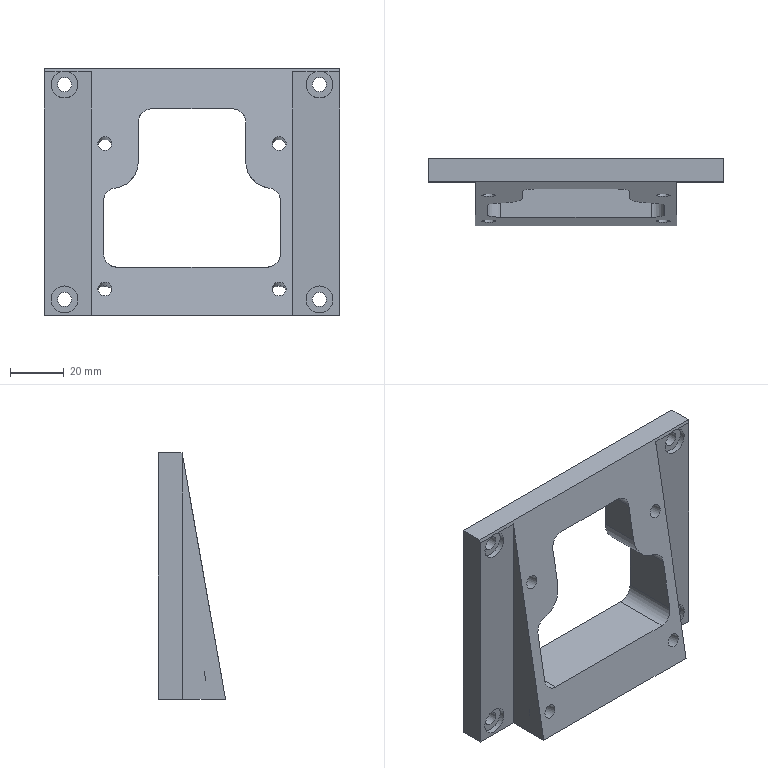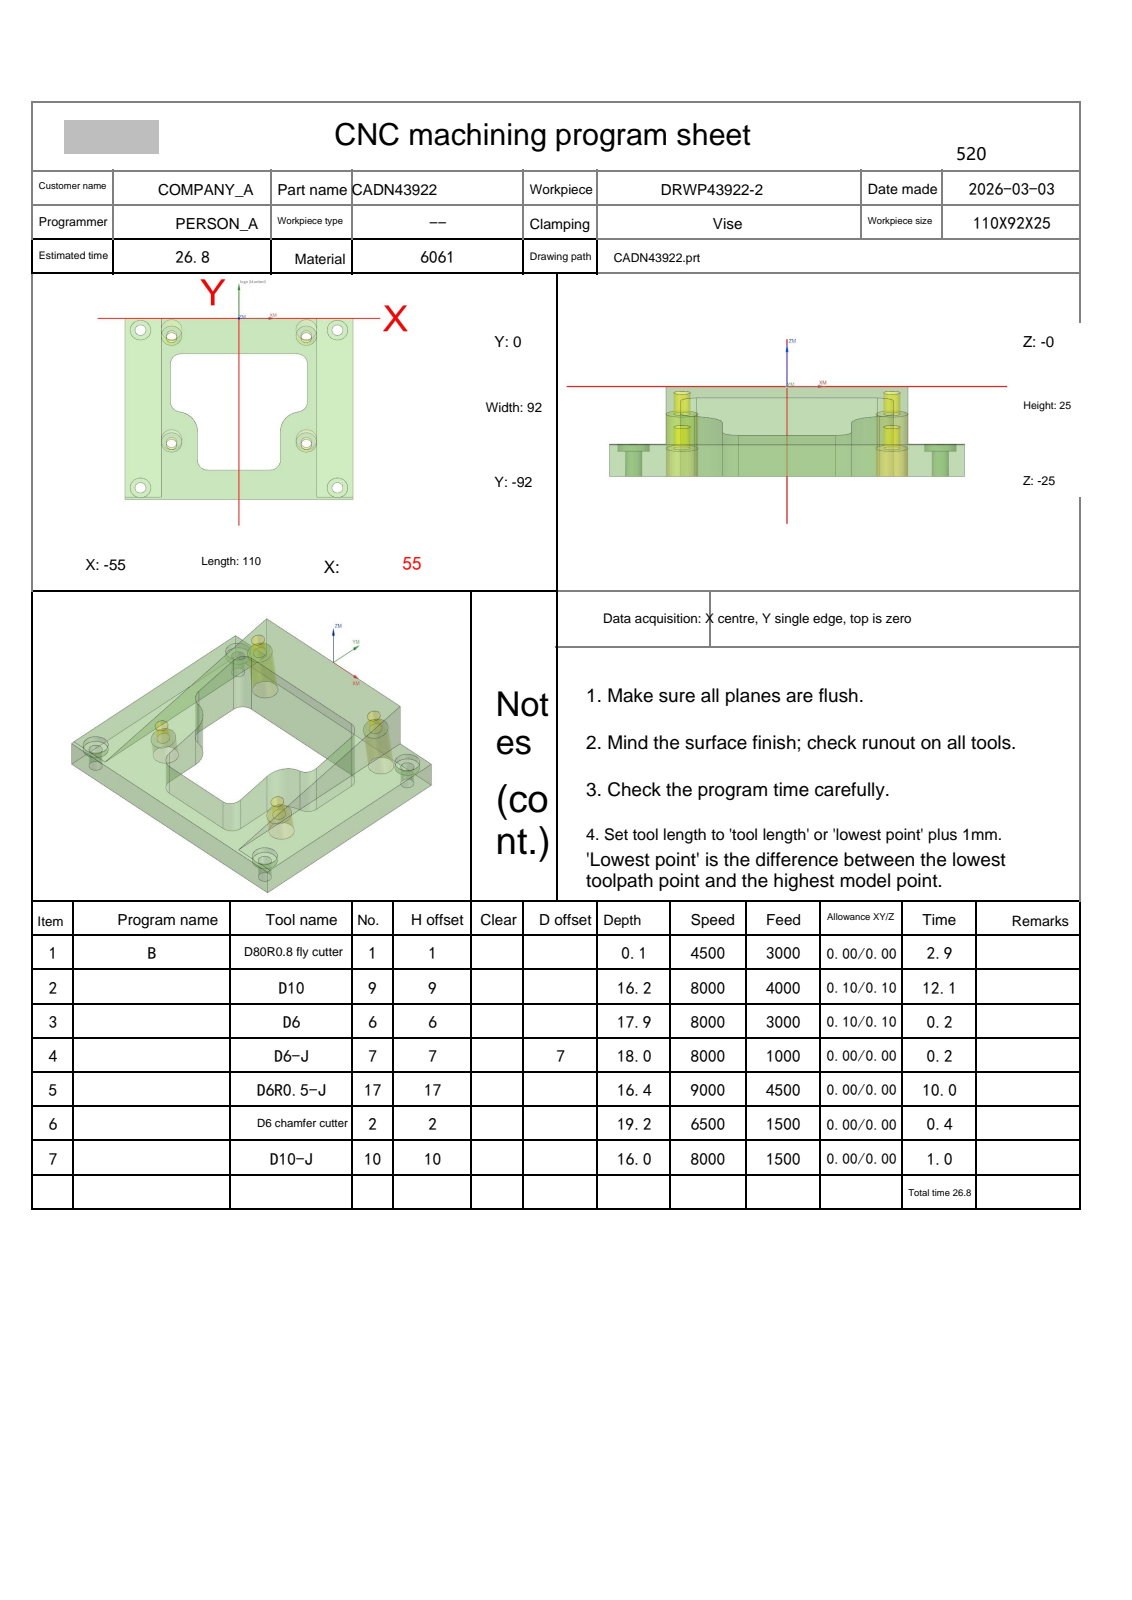NC program | NX | posted by the shop | part box 110 x 25 x 92 mm
Lines 1 to 182 of 14355:
%
O0001
(Machine time: 28.14 MIN)
(===Total Tool:7===)
(T1=D80R0.8 fly cutter D=80.  R=0.8  D-  H01 Z=0.    )
(T9=D10     D=10.  R=0.   D-  H09 Z=-16.22)
(T6=D6      D=6.   R=0.   D-  H06 Z=-17.9 )
(T7=D6-J    D=6.   R=0.   D7  H07 Z=-18.  )
(T17=D6R0.5-J D=6.   R=0.5  D-  H17 Z=-16.41)
(T2=D6 chamfer cutter   D=6.   R=0.   D-  H02 Z=-19.2 )
(T10=D10-J  D=10.  R=0.   D10 H10 Z=-16.  )
G80 G90 G17 G49 G40
G91 G28 Z0
M01
N1 T01 M06
(D80R0.8 fly cutter  D=80. R=0.8 H=01 ce=0.20 di=0.10)
G00 G90 G54 X-107. Y-3. M03 S4500
G43 H01 Z50.
M08
Z6.011
G01 Z4.011 F3000.
X-95.
X87.8
G02 X95. Y-10.2 I0.0 J-7.2
G01 Y-38.8
G02 X87.8 Y-46. I-7.2 J0.0
G01 X-87.8
G03 X-95. Y-53.2 I0.0 J-7.2
G01 Y-81.8
G03 X-87.8 Y-89. I7.2 J0.0
G01 X95.
X107.
Z6.011
G00 Z7.5
X-107. Y-3.
Z5.522
G01 Z3.522
X-95.
X87.8
G02 X95. Y-10.2 I0.0 J-7.2
G01 Y-38.8
G02 X87.8 Y-46. I-7.2 J0.0
G01 X-87.8
G03 X-95. Y-53.2 I0.0 J-7.2
G01 Y-81.8
G03 X-87.8 Y-89. I7.2 J0.0
G01 X95.
X107.
Z5.522
G00 Z7.011
X-107. Y-3.
Z5.033
G01 Z3.033
X-95.
X87.8
G02 X95. Y-10.2 I0.0 J-7.2
G01 Y-38.8
G02 X87.8 Y-46. I-7.2 J0.0
G01 X-87.8
G03 X-95. Y-53.2 I0.0 J-7.2
G01 Y-81.8
G03 X-87.8 Y-89. I7.2 J0.0
G01 X95.
X107.
Z5.033
G00 Z6.522
X-107. Y-3.
Z4.544
G01 Z2.544
X-95.
X87.8
G02 X95. Y-10.2 I0.0 J-7.2
G01 Y-38.8
G02 X87.8 Y-46. I-7.2 J0.0
G01 X-87.8
G03 X-95. Y-53.2 I0.0 J-7.2
G01 Y-81.8
G03 X-87.8 Y-89. I7.2 J0.0
G01 X95.
X107.
Z4.544
G00 Z6.033
X-107. Y-3.
Z4.056
G01 Z2.056
X-95.
X87.8
G02 X95. Y-10.2 I0.0 J-7.2
G01 Y-38.8
G02 X87.8 Y-46. I-7.2 J0.0
G01 X-87.8
G03 X-95. Y-53.2 I0.0 J-7.2
G01 Y-81.8
G03 X-87.8 Y-89. I7.2 J0.0
G01 X95.
X107.
Z4.056
G00 Z5.544
X-107. Y-3.
Z3.567
G01 Z1.567
X-95.
X87.8
G02 X95. Y-10.2 I0.0 J-7.2
G01 Y-38.8
G02 X87.8 Y-46. I-7.2 J0.0
G01 X-87.8
G03 X-95. Y-53.2 I0.0 J-7.2
G01 Y-81.8
G03 X-87.8 Y-89. I7.2 J0.0
G01 X95.
X107.
Z3.567
G00 Z5.056
X-107. Y-3.
Z3.078
G01 Z1.078
X-95.
X87.8
G02 X95. Y-10.2 I0.0 J-7.2
G01 Y-38.8
G02 X87.8 Y-46. I-7.2 J0.0
G01 X-87.8
G03 X-95. Y-53.2 I0.0 J-7.2
G01 Y-81.8
G03 X-87.8 Y-89. I7.2 J0.0
G01 X95.
X107.
Z3.078
G00 Z4.567
X-107. Y-3.
Z2.589
G01 Z.589
X-95.
X87.8
G02 X95. Y-10.2 I0.0 J-7.2
G01 Y-38.8
G02 X87.8 Y-46. I-7.2 J0.0
G01 X-87.8
G03 X-95. Y-53.2 I0.0 J-7.2
G01 Y-81.8
G03 X-87.8 Y-89. I7.2 J0.0
G01 X95.
X107.
Z2.589
G00 Z4.078
X-107. Y-3.
Z2.1
G01 Z.1
X-95.
X87.8
G02 X95. Y-10.2 I0.0 J-7.2
G01 Y-38.8
G02 X87.8 Y-46. I-7.2 J0.0
G01 X-87.8
G03 X-95. Y-53.2 I0.0 J-7.2
G01 Y-81.8
G03 X-87.8 Y-89. I7.2 J0.0
G01 X95.
X107.
Z2.1
G00 Z50.
G00 G90 X-107. Y-3. M03 S4500
Z50.
Z2.
G01 Z0.0 F1000.
X-95.
X95.
Y-46.
X-95.
Y-89.
X95.
X107.
Z2.
G00 Z50.
G91 G28 Z0.0
M05
M09
G91 G28 Z0.0
M01